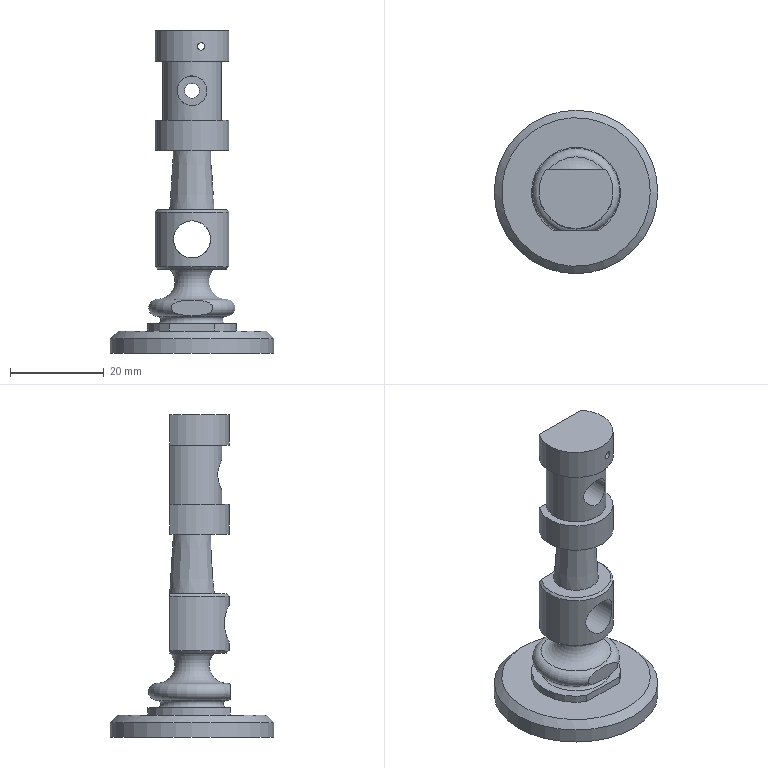Part | NX | features DATUM_CSYS 9, SKETCH 8, EXTRUDE 5, CYLINDER 4, SWP104 3, CHAMFER 2, Intersection Curve 2, CPROJ 1 | 1 solid | 33 faces | box 34.925 x 34.925 x 68.955 mm | volume 12101 mm3 | plane 15 | cylinder 11 | cone 4 | torus 3 | commonest cylinder face diameters 15.875 x3 1.587 x2 3.175 x1 6.35 x1 7.938 x1 12.7 x1
STEP:
#1=CARTESIAN_POINT('',(0.,-7.493,6.35));
#2=VERTEX_POINT('',#1);
#3=CARTESIAN_POINT('',(0.,0.,6.35));
#4=DIRECTION('',(0.,0.,1.));
#5=DIRECTION('',(0.,-1.,0.));
#6=AXIS2_PLACEMENT_3D('',#3,#4,#5);
#7=CIRCLE('',#6,7.493);
#8=EDGE_CURVE('',#2,#2,#7,.T.);
#9=ORIENTED_EDGE('',*,*,#8,.F.);
#10=EDGE_LOOP('',(#9));
#11=FACE_BOUND('',#10,.T.);
#12=CARTESIAN_POINT('',(-4.897,-8.169,6.35));
#13=VERTEX_POINT('',#12);
#14=CARTESIAN_POINT('',(4.897,-8.169,6.35));
#15=VERTEX_POINT('',#14);
#16=CARTESIAN_POINT('',(0.,0.,6.35));
#17=DIRECTION('',(0.,0.,-1.));
#18=DIRECTION('',(1.,0.,0.));
#19=AXIS2_PLACEMENT_3D('',#16,#17,#18);
#20=CIRCLE('',#19,9.525);
#21=EDGE_CURVE('',#13,#15,#20,.T.);
#22=ORIENTED_EDGE('',*,*,#21,.F.);
#23=CARTESIAN_POINT('',(0.,-8.169,6.35));
#24=DIRECTION('',(1.,0.,0.));
#25=VECTOR('',#24,1000.);
#26=LINE('',#23,#25);
#27=EDGE_CURVE('',#13,#15,#26,.T.);
#28=ORIENTED_EDGE('',*,*,#27,.T.);
#29=EDGE_LOOP('',(#22,#28));
#30=FACE_BOUND('',#29,.T.);
#31=CARTESIAN_POINT('',(0.,0.,6.35));
#32=DIRECTION('',(0.,0.,1.));
#33=DIRECTION('',(1.,0.,0.));
#34=AXIS2_PLACEMENT_3D('',#31,#32,#33);
#35=PLANE('',#34);
#36=ADVANCED_FACE('',(#11,#30),#35,.T.);
#37=ORIENTED_EDGE('',*,*,#21,.T.);
#38=CARTESIAN_POINT('',(4.897,-8.169,4.762));
#39=VERTEX_POINT('',#38);
#40=CARTESIAN_POINT('',(4.897,-8.169,4.762));
#41=DIRECTION('',(0.,0.,1.));
#42=VECTOR('',#41,1000.);
#43=LINE('',#40,#42);
#44=EDGE_CURVE('',#15,#39,#43,.F.);
#45=ORIENTED_EDGE('',*,*,#44,.T.);
#46=CARTESIAN_POINT('',(-4.897,-8.169,4.762));
#47=VERTEX_POINT('',#46);
#48=CARTESIAN_POINT('',(0.,0.,4.763));
#49=DIRECTION('',(0.,0.,1.));
#50=DIRECTION('',(1.,0.,0.));
#51=AXIS2_PLACEMENT_3D('',#48,#49,#50);
#52=CIRCLE('',#51,9.525);
#53=EDGE_CURVE('',#39,#47,#52,.T.);
#54=ORIENTED_EDGE('',*,*,#53,.T.);
#55=CARTESIAN_POINT('',(-4.897,-8.169,4.762));
#56=DIRECTION('',(0.,0.,1.));
#57=VECTOR('',#56,1000.);
#58=LINE('',#55,#57);
#59=EDGE_CURVE('',#47,#13,#58,.T.);
#60=ORIENTED_EDGE('',*,*,#59,.T.);
#61=EDGE_LOOP('',(#37,#45,#54,#60));
#62=FACE_BOUND('',#61,.T.);
#63=CARTESIAN_POINT('',(0.,0.,4.763));
#64=DIRECTION('',(0.,0.,1.));
#65=DIRECTION('',(1.,0.,0.));
#66=AXIS2_PLACEMENT_3D('',#63,#64,#65);
#67=CYLINDRICAL_SURFACE('',#66,9.525);
#68=ADVANCED_FACE('',(#62),#67,.T.);
#69=CARTESIAN_POINT('',(0.,-7.493,7.937));
#70=VERTEX_POINT('',#69);
#71=CARTESIAN_POINT('',(0.,0.,7.937));
#72=DIRECTION('',(0.,0.,1.));
#73=DIRECTION('',(0.,-1.,0.));
#74=AXIS2_PLACEMENT_3D('',#71,#72,#73);
#75=CIRCLE('',#74,7.493);
#76=EDGE_CURVE('',#70,#70,#75,.T.);
#77=ORIENTED_EDGE('',*,*,#76,.T.);
#78=EDGE_LOOP('',(#77));
#79=FACE_BOUND('',#78,.T.);
#80=CARTESIAN_POINT('',(0.,7.493,11.537));
#81=VERTEX_POINT('',#80);
#82=CARTESIAN_POINT('',(0.,0.,11.537));
#83=DIRECTION('',(0.,0.,-1.));
#84=DIRECTION('',(0.,1.,0.));
#85=AXIS2_PLACEMENT_3D('',#82,#83,#84);
#86=CIRCLE('',#85,7.493);
#87=EDGE_CURVE('',#81,#81,#86,.T.);
#88=ORIENTED_EDGE('',*,*,#87,.T.);
#89=EDGE_LOOP('',(#88));
#90=FACE_BOUND('',#89,.T.);
#91=CARTESIAN_POINT('',(0.,-8.169,8.069));
#92=VERTEX_POINT('',#91);
#93=CARTESIAN_POINT('',(1.27,-8.169,8.094));
#94=CARTESIAN_POINT('',(0.001629,-8.169,8.057));
#95=CARTESIAN_POINT('',(-1.276,-8.169,8.094));
#96=CARTESIAN_POINT('',(-2.544,-8.169,8.244));
#97=CARTESIAN_POINT('',(-3.572,-8.169,8.567));
#98=CARTESIAN_POINT('',(-4.256,-8.169,9.104));
#99=CARTESIAN_POINT('',(-4.518,-8.169,9.743));
#100=CARTESIAN_POINT('',(-4.25,-8.169,10.378));
#101=CARTESIAN_POINT('',(-3.558,-8.169,10.915));
#102=CARTESIAN_POINT('',(-2.519,-8.169,11.235));
#103=CARTESIAN_POINT('',(-1.257,-8.169,11.382));
#104=CARTESIAN_POINT('',(0.01726,-8.169,11.418));
#105=CARTESIAN_POINT('',(1.296,-8.169,11.38));
#106=CARTESIAN_POINT('',(2.566,-8.169,11.226));
#107=CARTESIAN_POINT('',(3.593,-8.169,10.899));
#108=CARTESIAN_POINT('',(4.27,-8.169,10.352));
#109=CARTESIAN_POINT('',(4.515,-8.169,9.717));
#110=CARTESIAN_POINT('',(4.243,-8.169,9.091));
#111=CARTESIAN_POINT('',(3.558,-8.169,8.562));
#112=CARTESIAN_POINT('',(2.53,-8.169,8.242));
#113=CARTESIAN_POINT('',(1.27,-8.169,8.094));
#114=CARTESIAN_POINT('',(0.001629,-8.169,8.057));
#115=CARTESIAN_POINT('',(-1.276,-8.169,8.094));
#116=B_SPLINE_CURVE_WITH_KNOTS('',3,(#93,#94,#95,#96,#97,#98,#99,#100,#101,#102,#103,#104,#105,#106,#107,#108,#109,#110,#111,#112,#113,#114,#115),.UNSPECIFIED.,.T.,.F.,(1,1,1,1,1,1,1,1,1,1,1,1,1,1,1,1,1,1,1,1,1,1,1,1,1,1,1),(-0.003821,-0.002548,-0.001274,0.,0.001274,0.002548,0.003821,0.004458,0.005095,0.005732,0.006369,0.007643,0.008916,0.01019,0.01146,0.01274,0.01401,0.01465,0.01529,0.01592,0.01656,0.01783,0.01911,0.02038,0.02165,0.02293,0.0242),.UNSPECIFIED.);
#117=EDGE_CURVE('',#92,#92,#116,.T.);
#118=ORIENTED_EDGE('',*,*,#117,.T.);
#119=EDGE_LOOP('',(#118));
#120=FACE_BOUND('',#119,.T.);
#121=CARTESIAN_POINT('',(0.,0.,9.737));
#122=DIRECTION('',(0.,0.,-1.));
#123=DIRECTION('',(0.,1.,0.));
#124=AXIS2_PLACEMENT_3D('',#121,#122,#123);
#125=TOROIDAL_SURFACE('',#124,7.493,1.8);
#126=ADVANCED_FACE('',(#79,#90,#120),#125,.T.);
#127=CARTESIAN_POINT('',(0.,4.763,18.005));
#128=VERTEX_POINT('',#127);
#129=CARTESIAN_POINT('',(5.713,4.763,18.005));
#130=VERTEX_POINT('',#129);
#131=CARTESIAN_POINT('',(0.,4.763,18.005));
#132=DIRECTION('',(1.,0.,0.));
#133=VECTOR('',#132,1000.);
#134=LINE('',#131,#133);
#135=EDGE_CURVE('',#128,#130,#134,.T.);
#136=ORIENTED_EDGE('',*,*,#135,.T.);
#137=CARTESIAN_POINT('',(-5.713,4.763,18.005));
#138=VERTEX_POINT('',#137);
#139=CARTESIAN_POINT('',(0.,0.,18.005));
#140=DIRECTION('',(0.,0.,-1.));
#141=DIRECTION('',(0.,1.,0.));
#142=AXIS2_PLACEMENT_3D('',#139,#140,#141);
#143=CIRCLE('',#142,7.438);
#144=EDGE_CURVE('',#130,#138,#143,.T.);
#145=ORIENTED_EDGE('',*,*,#144,.T.);
#146=CARTESIAN_POINT('',(0.,4.763,18.005));
#147=DIRECTION('',(1.,0.,0.));
#148=VECTOR('',#147,1000.);
#149=LINE('',#146,#148);
#150=EDGE_CURVE('',#138,#128,#149,.T.);
#151=ORIENTED_EDGE('',*,*,#150,.T.);
#152=CARTESIAN_POINT('',(0.,0.,18.005));
#153=DIRECTION('',(0.,0.,1.));
#154=DIRECTION('',(0.,-1.,0.));
#155=AXIS2_PLACEMENT_3D('',#152,#153,#154);
#156=CIRCLE('',#155,4.763);
#157=EDGE_CURVE('',#128,#128,#156,.T.);
#158=ORIENTED_EDGE('',*,*,#157,.T.);
#159=EDGE_LOOP('',(#136,#145,#151,#158));
#160=FACE_BOUND('',#159,.T.);
#161=CARTESIAN_POINT('',(0.,0.,18.005));
#162=DIRECTION('',(0.,0.,-1.));
#163=DIRECTION('',(0.,1.,0.));
#164=AXIS2_PLACEMENT_3D('',#161,#162,#163);
#165=PLANE('',#164);
#166=ADVANCED_FACE('',(#160),#165,.T.);
#167=CARTESIAN_POINT('',(0.,-7.938,28.323));
#168=VERTEX_POINT('',#167);
#169=CARTESIAN_POINT('',(3.118,-7.441,27.461));
#170=CARTESIAN_POINT('',(-0.001391,-8.185,28.755));
#171=CARTESIAN_POINT('',(-3.112,-7.443,27.458));
#172=CARTESIAN_POINT('',(-4.396,-6.59,24.369));
#173=CARTESIAN_POINT('',(-3.115,-7.44,21.25));
#174=CARTESIAN_POINT('',(-0.01564,-8.185,19.955));
#175=CARTESIAN_POINT('',(3.112,-7.445,21.246));
#176=CARTESIAN_POINT('',(4.396,-6.59,24.34));
#177=CARTESIAN_POINT('',(3.118,-7.441,27.461));
#178=CARTESIAN_POINT('',(-0.001391,-8.185,28.755));
#179=CARTESIAN_POINT('',(-3.112,-7.443,27.458));
#180=B_SPLINE_CURVE_WITH_KNOTS('',3,(#169,#170,#171,#172,#173,#174,#175,#176,#177,#178,#179),.UNSPECIFIED.,.T.,.F.,(1,1,1,1,1,1,1,1,1,1,1,1,1,1,1),(-0.00946,-0.006307,-0.003153,0.,0.003153,0.006307,0.00946,0.01261,0.01577,0.01892,0.02207,0.02523,0.02838,0.03153,0.03469),.UNSPECIFIED.);
#181=EDGE_CURVE('',#168,#168,#180,.T.);
#182=ORIENTED_EDGE('',*,*,#181,.F.);
#183=EDGE_LOOP('',(#182));
#184=FACE_BOUND('',#183,.T.);
#185=CARTESIAN_POINT('',(-6.35,4.763,30.205));
#186=VERTEX_POINT('',#185);
#187=CARTESIAN_POINT('',(-6.35,4.762,18.505));
#188=VERTEX_POINT('',#187);
#189=CARTESIAN_POINT('',(-6.35,4.763,43.405));
#190=DIRECTION('',(0.,0.,-1.));
#191=VECTOR('',#190,1000.);
#192=LINE('',#189,#191);
#193=EDGE_CURVE('',#186,#188,#192,.T.);
#194=ORIENTED_EDGE('',*,*,#193,.T.);
#195=CARTESIAN_POINT('',(6.35,4.762,18.505));
#196=VERTEX_POINT('',#195);
#197=CARTESIAN_POINT('',(0.,0.,18.505));
#198=DIRECTION('',(0.,0.,-1.));
#199=DIRECTION('',(0.,1.,0.));
#200=AXIS2_PLACEMENT_3D('',#197,#198,#199);
#201=CIRCLE('',#200,7.938);
#202=EDGE_CURVE('',#188,#196,#201,.F.);
#203=ORIENTED_EDGE('',*,*,#202,.T.);
#204=CARTESIAN_POINT('',(6.35,4.763,30.205));
#205=VERTEX_POINT('',#204);
#206=CARTESIAN_POINT('',(6.35,4.763,43.405));
#207=DIRECTION('',(0.,0.,-1.));
#208=VECTOR('',#207,1000.);
#209=LINE('',#206,#208);
#210=EDGE_CURVE('',#196,#205,#209,.F.);
#211=ORIENTED_EDGE('',*,*,#210,.T.);
#212=CARTESIAN_POINT('',(0.,0.,30.205));
#213=DIRECTION('',(0.,0.,1.));
#214=DIRECTION('',(0.,-1.,0.));
#215=AXIS2_PLACEMENT_3D('',#212,#213,#214);
#216=CIRCLE('',#215,7.938);
#217=EDGE_CURVE('',#205,#186,#216,.F.);
#218=ORIENTED_EDGE('',*,*,#217,.T.);
#219=EDGE_LOOP('',(#194,#203,#211,#218));
#220=FACE_BOUND('',#219,.T.);
#221=CARTESIAN_POINT('',(0.,0.,43.405));
#222=DIRECTION('',(0.,0.,-1.));
#223=DIRECTION('',(0.,1.,0.));
#224=AXIS2_PLACEMENT_3D('',#221,#222,#223);
#225=CYLINDRICAL_SURFACE('',#224,7.938);
#226=ADVANCED_FACE('',(#184,#220),#225,.T.);
#227=CARTESIAN_POINT('',(0.,4.763,30.705));
#228=VERTEX_POINT('',#227);
#229=CARTESIAN_POINT('',(-5.713,4.763,30.705));
#230=VERTEX_POINT('',#229);
#231=CARTESIAN_POINT('',(0.,4.763,30.705));
#232=DIRECTION('',(-1.,0.,0.));
#233=VECTOR('',#232,1000.);
#234=LINE('',#231,#233);
#235=EDGE_CURVE('',#228,#230,#234,.T.);
#236=ORIENTED_EDGE('',*,*,#235,.T.);
#237=CARTESIAN_POINT('',(5.713,4.763,30.705));
#238=VERTEX_POINT('',#237);
#239=CARTESIAN_POINT('',(0.,0.,30.705));
#240=DIRECTION('',(0.,0.,1.));
#241=DIRECTION('',(0.,-1.,0.));
#242=AXIS2_PLACEMENT_3D('',#239,#240,#241);
#243=CIRCLE('',#242,7.438);
#244=EDGE_CURVE('',#230,#238,#243,.T.);
#245=ORIENTED_EDGE('',*,*,#244,.T.);
#246=CARTESIAN_POINT('',(0.,4.763,30.705));
#247=DIRECTION('',(-1.,0.,0.));
#248=VECTOR('',#247,1000.);
#249=LINE('',#246,#248);
#250=EDGE_CURVE('',#238,#228,#249,.T.);
#251=ORIENTED_EDGE('',*,*,#250,.T.);
#252=CARTESIAN_POINT('',(0.,0.,30.705));
#253=DIRECTION('',(0.,0.,-1.));
#254=DIRECTION('',(0.,1.,0.));
#255=AXIS2_PLACEMENT_3D('',#252,#253,#254);
#256=CIRCLE('',#255,4.763);
#257=EDGE_CURVE('',#228,#228,#256,.T.);
#258=ORIENTED_EDGE('',*,*,#257,.T.);
#259=EDGE_LOOP('',(#236,#245,#251,#258));
#260=FACE_BOUND('',#259,.T.);
#261=CARTESIAN_POINT('',(0.,7.938,30.705));
#262=DIRECTION('',(0.,0.,1.));
#263=DIRECTION('',(0.,-1.,0.));
#264=AXIS2_PLACEMENT_3D('',#261,#262,#263);
#265=PLANE('',#264);
#266=ADVANCED_FACE('',(#260),#265,.T.);
#267=CARTESIAN_POINT('',(0.,3.969,43.405));
#268=VERTEX_POINT('',#267);
#269=CARTESIAN_POINT('',(0.,0.,43.405));
#270=DIRECTION('',(0.,0.,-1.));
#271=DIRECTION('',(0.,1.,0.));
#272=AXIS2_PLACEMENT_3D('',#269,#270,#271);
#273=CIRCLE('',#272,3.969);
#274=EDGE_CURVE('',#268,#268,#273,.T.);
#275=ORIENTED_EDGE('',*,*,#274,.F.);
#276=EDGE_LOOP('',(#275));
#277=FACE_BOUND('',#276,.T.);
#278=CARTESIAN_POINT('',(6.35,4.763,43.405));
#279=VERTEX_POINT('',#278);
#280=CARTESIAN_POINT('',(-6.35,4.763,43.405));
#281=VERTEX_POINT('',#280);
#282=CARTESIAN_POINT('',(0.,0.,43.405));
#283=DIRECTION('',(0.,0.,-1.));
#284=DIRECTION('',(0.,1.,0.));
#285=AXIS2_PLACEMENT_3D('',#282,#283,#284);
#286=CIRCLE('',#285,7.938);
#287=EDGE_CURVE('',#279,#281,#286,.T.);
#288=ORIENTED_EDGE('',*,*,#287,.T.);
#289=CARTESIAN_POINT('',(0.,4.763,43.405));
#290=DIRECTION('',(1.,0.,0.));
#291=VECTOR('',#290,1000.);
#292=LINE('',#289,#291);
#293=EDGE_CURVE('',#281,#279,#292,.T.);
#294=ORIENTED_EDGE('',*,*,#293,.T.);
#295=EDGE_LOOP('',(#288,#294));
#296=FACE_BOUND('',#295,.T.);
#297=CARTESIAN_POINT('',(0.,3.969,43.405));
#298=DIRECTION('',(0.,0.,-1.));
#299=DIRECTION('',(0.,1.,0.));
#300=AXIS2_PLACEMENT_3D('',#297,#298,#299);
#301=PLANE('',#300);
#302=ADVANCED_FACE('',(#277,#296),#301,.T.);
#303=ORIENTED_EDGE('',*,*,#287,.F.);
#304=CARTESIAN_POINT('',(6.35,4.762,49.755));
#305=VERTEX_POINT('',#304);
#306=CARTESIAN_POINT('',(6.35,4.763,43.405));
#307=DIRECTION('',(0.,0.,-1.));
#308=VECTOR('',#307,1000.);
#309=LINE('',#306,#308);
#310=EDGE_CURVE('',#279,#305,#309,.F.);
#311=ORIENTED_EDGE('',*,*,#310,.T.);
#312=CARTESIAN_POINT('',(-6.35,4.762,49.755));
#313=VERTEX_POINT('',#312);
#314=CARTESIAN_POINT('',(0.,0.,49.755));
#315=DIRECTION('',(0.,0.,-1.));
#316=DIRECTION('',(0.,1.,0.));
#317=AXIS2_PLACEMENT_3D('',#314,#315,#316);
#318=CIRCLE('',#317,7.938);
#319=EDGE_CURVE('',#305,#313,#318,.T.);
#320=ORIENTED_EDGE('',*,*,#319,.T.);
#321=CARTESIAN_POINT('',(-6.35,4.763,43.405));
#322=DIRECTION('',(0.,0.,-1.));
#323=VECTOR('',#322,1000.);
#324=LINE('',#321,#323);
#325=EDGE_CURVE('',#313,#281,#324,.T.);
#326=ORIENTED_EDGE('',*,*,#325,.T.);
#327=EDGE_LOOP('',(#303,#311,#320,#326));
#328=FACE_BOUND('',#327,.T.);
#329=CARTESIAN_POINT('',(0.,0.,43.405));
#330=DIRECTION('',(0.,0.,-1.));
#331=DIRECTION('',(0.,1.,0.));
#332=AXIS2_PLACEMENT_3D('',#329,#330,#331);
#333=CYLINDRICAL_SURFACE('',#332,7.938);
#334=ADVANCED_FACE('',(#328),#333,.T.);
#335=ORIENTED_EDGE('',*,*,#319,.F.);
#336=CARTESIAN_POINT('',(4.2,4.763,49.755));
#337=VERTEX_POINT('',#336);
#338=CARTESIAN_POINT('',(0.,4.762,49.755));
#339=DIRECTION('',(-1.,0.,0.));
#340=VECTOR('',#339,1000.);
#341=LINE('',#338,#340);
#342=EDGE_CURVE('',#305,#337,#341,.T.);
#343=ORIENTED_EDGE('',*,*,#342,.T.);
#344=CARTESIAN_POINT('',(-4.2,4.763,49.755));
#345=VERTEX_POINT('',#344);
#346=CARTESIAN_POINT('',(0.,0.,49.755));
#347=DIRECTION('',(0.,0.,-1.));
#348=DIRECTION('',(0.,1.,0.));
#349=AXIS2_PLACEMENT_3D('',#346,#347,#348);
#350=CIRCLE('',#349,6.35);
#351=EDGE_CURVE('',#337,#345,#350,.T.);
#352=ORIENTED_EDGE('',*,*,#351,.T.);
#353=CARTESIAN_POINT('',(0.,4.762,49.755));
#354=DIRECTION('',(-1.,0.,0.));
#355=VECTOR('',#354,1000.);
#356=LINE('',#353,#355);
#357=EDGE_CURVE('',#345,#313,#356,.T.);
#358=ORIENTED_EDGE('',*,*,#357,.T.);
#359=EDGE_LOOP('',(#335,#343,#352,#358));
#360=FACE_BOUND('',#359,.T.);
#361=CARTESIAN_POINT('',(0.,7.938,49.755));
#362=DIRECTION('',(0.,0.,1.));
#363=DIRECTION('',(0.,-1.,0.));
#364=AXIS2_PLACEMENT_3D('',#361,#362,#363);
#365=PLANE('',#364);
#366=ADVANCED_FACE('',(#360),#365,.T.);
#367=CARTESIAN_POINT('',(3.175,-5.499,56.105));
#368=VERTEX_POINT('',#367);
#369=CARTESIAN_POINT('',(2.491,-5.955,53.617));
#370=CARTESIAN_POINT('',(3.517,-5.272,56.106));
#371=CARTESIAN_POINT('',(2.489,-5.954,58.588));
#372=CARTESIAN_POINT('',(0.009887,-6.548,59.625));
#373=CARTESIAN_POINT('',(-2.49,-5.955,58.59));
#374=CARTESIAN_POINT('',(-3.517,-5.272,56.117));
#375=CARTESIAN_POINT('',(-2.493,-5.952,53.621));
#376=CARTESIAN_POINT('',(-0.01032,-6.548,52.585));
#377=CARTESIAN_POINT('',(2.491,-5.955,53.617));
#378=CARTESIAN_POINT('',(3.517,-5.272,56.106));
#379=CARTESIAN_POINT('',(2.489,-5.954,58.588));
#380=B_SPLINE_CURVE_WITH_KNOTS('',3,(#369,#370,#371,#372,#373,#374,#375,#376,#377,#378,#379),.UNSPECIFIED.,.T.,.F.,(1,1,1,1,1,1,1,1,1,1,1,1,1,1,1),(-0.007567,-0.005045,-0.002522,0.,0.002522,0.005045,0.007567,0.01009,0.01261,0.01513,0.01766,0.02018,0.0227,0.02522,0.02775),.UNSPECIFIED.);
#381=EDGE_CURVE('',#368,#368,#380,.T.);
#382=ORIENTED_EDGE('',*,*,#381,.F.);
#383=EDGE_LOOP('',(#382));
#384=FACE_BOUND('',#383,.T.);
#385=ORIENTED_EDGE('',*,*,#351,.F.);
#386=CARTESIAN_POINT('',(4.2,4.762,62.455));
#387=VERTEX_POINT('',#386);
#388=CARTESIAN_POINT('',(4.2,4.763,43.405));
#389=DIRECTION('',(0.,0.,-1.));
#390=VECTOR('',#389,1000.);
#391=LINE('',#388,#390);
#392=EDGE_CURVE('',#337,#387,#391,.F.);
#393=ORIENTED_EDGE('',*,*,#392,.T.);
#394=CARTESIAN_POINT('',(-4.2,4.762,62.455));
#395=VERTEX_POINT('',#394);
#396=CARTESIAN_POINT('',(0.,0.,62.455));
#397=DIRECTION('',(0.,0.,-1.));
#398=DIRECTION('',(0.,1.,0.));
#399=AXIS2_PLACEMENT_3D('',#396,#397,#398);
#400=CIRCLE('',#399,6.35);
#401=EDGE_CURVE('',#387,#395,#400,.T.);
#402=ORIENTED_EDGE('',*,*,#401,.T.);
#403=CARTESIAN_POINT('',(-4.2,4.763,43.405));
#404=DIRECTION('',(0.,0.,-1.));
#405=VECTOR('',#404,1000.);
#406=LINE('',#403,#405);
#407=EDGE_CURVE('',#395,#345,#406,.T.);
#408=ORIENTED_EDGE('',*,*,#407,.T.);
#409=EDGE_LOOP('',(#385,#393,#402,#408));
#410=FACE_BOUND('',#409,.T.);
#411=CARTESIAN_POINT('',(0.,0.,43.405));
#412=DIRECTION('',(0.,0.,-1.));
#413=DIRECTION('',(0.,1.,0.));
#414=AXIS2_PLACEMENT_3D('',#411,#412,#413);
#415=CYLINDRICAL_SURFACE('',#414,6.35);
#416=ADVANCED_FACE('',(#384,#410),#415,.T.);
#417=CARTESIAN_POINT('',(6.35,4.763,62.455));
#418=VERTEX_POINT('',#417);
#419=CARTESIAN_POINT('',(-6.35,4.763,62.455));
#420=VERTEX_POINT('',#419);
#421=CARTESIAN_POINT('',(0.,0.,62.455));
#422=DIRECTION('',(0.,0.,-1.));
#423=DIRECTION('',(0.,1.,0.));
#424=AXIS2_PLACEMENT_3D('',#421,#422,#423);
#425=CIRCLE('',#424,7.938);
#426=EDGE_CURVE('',#418,#420,#425,.T.);
#427=ORIENTED_EDGE('',*,*,#426,.T.);
#428=CARTESIAN_POINT('',(0.,4.762,62.455));
#429=DIRECTION('',(1.,0.,0.));
#430=VECTOR('',#429,1000.);
#431=LINE('',#428,#430);
#432=EDGE_CURVE('',#420,#395,#431,.T.);
#433=ORIENTED_EDGE('',*,*,#432,.T.);
#434=ORIENTED_EDGE('',*,*,#401,.F.);
#435=CARTESIAN_POINT('',(0.,4.762,62.455));
#436=DIRECTION('',(1.,0.,0.));
#437=VECTOR('',#436,1000.);
#438=LINE('',#435,#437);
#439=EDGE_CURVE('',#387,#418,#438,.T.);
#440=ORIENTED_EDGE('',*,*,#439,.T.);
#441=EDGE_LOOP('',(#427,#433,#434,#440));
#442=FACE_BOUND('',#441,.T.);
#443=CARTESIAN_POINT('',(0.,6.35,62.455));
#444=DIRECTION('',(0.,0.,-1.));
#445=DIRECTION('',(0.,1.,0.));
#446=AXIS2_PLACEMENT_3D('',#443,#444,#445);
#447=PLANE('',#446);
#448=ADVANCED_FACE('',(#442),#447,.T.);
#449=CARTESIAN_POINT('',(1.903,-7.706,66.381));
#450=VERTEX_POINT('',#449);
#451=CARTESIAN_POINT('',(2.515,-7.534,66.216));
#452=CARTESIAN_POINT('',(1.694,-7.779,66.558));
#453=CARTESIAN_POINT('',(0.9196,-7.885,65.803));
#454=CARTESIAN_POINT('',(1.295,-7.836,64.948));
#455=CARTESIAN_POINT('',(1.92,-7.712,64.712));
#456=CARTESIAN_POINT('',(2.523,-7.531,64.965));
#457=CARTESIAN_POINT('',(2.786,-7.432,65.594));
#458=CARTESIAN_POINT('',(2.515,-7.534,66.216));
#459=CARTESIAN_POINT('',(1.694,-7.779,66.558));
#460=CARTESIAN_POINT('',(0.9196,-7.885,65.803));
#461=B_SPLINE_CURVE_WITH_KNOTS('',3,(#451,#452,#453,#454,#455,#456,#457,#458,#459,#460),.UNSPECIFIED.,.T.,.F.,(1,1,1,1,1,1,1,1,1,1,1,1,1,1),(-0.00189,-0.00126,-0.0006301,0.,0.00126,0.00189,0.00252,0.003151,0.003781,0.004411,0.005041,0.006301,0.006931,0.007561),.UNSPECIFIED.);
#462=EDGE_CURVE('',#450,#450,#461,.T.);
#463=ORIENTED_EDGE('',*,*,#462,.F.);
#464=EDGE_LOOP('',(#463));
#465=FACE_BOUND('',#464,.T.);
#466=ORIENTED_EDGE('',*,*,#426,.F.);
#467=CARTESIAN_POINT('',(6.35,4.762,68.955));
#468=VERTEX_POINT('',#467);
#469=CARTESIAN_POINT('',(6.35,4.763,43.405));
#470=DIRECTION('',(0.,0.,-1.));
#471=VECTOR('',#470,1000.);
#472=LINE('',#469,#471);
#473=EDGE_CURVE('',#418,#468,#472,.F.);
#474=ORIENTED_EDGE('',*,*,#473,.T.);
#475=CARTESIAN_POINT('',(-6.35,4.762,68.955));
#476=VERTEX_POINT('',#475);
#477=CARTESIAN_POINT('',(0.,0.,68.955));
#478=DIRECTION('',(0.,0.,-1.));
#479=DIRECTION('',(0.,1.,0.));
#480=AXIS2_PLACEMENT_3D('',#477,#478,#479);
#481=CIRCLE('',#480,7.938);
#482=EDGE_CURVE('',#468,#476,#481,.T.);
#483=ORIENTED_EDGE('',*,*,#482,.T.);
#484=CARTESIAN_POINT('',(-6.35,4.763,43.405));
#485=DIRECTION('',(0.,0.,-1.));
#486=VECTOR('',#485,1000.);
#487=LINE('',#484,#486);
#488=EDGE_CURVE('',#476,#420,#487,.T.);
#489=ORIENTED_EDGE('',*,*,#488,.T.);
#490=EDGE_LOOP('',(#466,#474,#483,#489));
#491=FACE_BOUND('',#490,.T.);
#492=CARTESIAN_POINT('',(0.,0.,43.405));
#493=DIRECTION('',(0.,0.,-1.));
#494=DIRECTION('',(0.,1.,0.));
#495=AXIS2_PLACEMENT_3D('',#492,#493,#494);
#496=CYLINDRICAL_SURFACE('',#495,7.938);
#497=ADVANCED_FACE('',(#465,#491),#496,.T.);
#498=ORIENTED_EDGE('',*,*,#482,.F.);
#499=CARTESIAN_POINT('',(0.,4.762,68.955));
#500=DIRECTION('',(-1.,0.,0.));
#501=VECTOR('',#500,1000.);
#502=LINE('',#499,#501);
#503=EDGE_CURVE('',#468,#476,#502,.T.);
#504=ORIENTED_EDGE('',*,*,#503,.T.);
#505=EDGE_LOOP('',(#498,#504));
#506=FACE_BOUND('',#505,.T.);
#507=CARTESIAN_POINT('',(0.,7.938,68.955));
#508=DIRECTION('',(0.,0.,1.));
#509=DIRECTION('',(0.,-1.,0.));
#510=AXIS2_PLACEMENT_3D('',#507,#508,#509);
#511=PLANE('',#510);
#512=ADVANCED_FACE('',(#506),#511,.T.);
#513=ORIENTED_EDGE('',*,*,#53,.F.);
#514=CARTESIAN_POINT('',(22.,-8.169,4.762));
#515=DIRECTION('',(-1.,0.,0.));
#516=VECTOR('',#515,1000.);
#517=LINE('',#514,#516);
#518=EDGE_CURVE('',#39,#47,#517,.T.);
#519=ORIENTED_EDGE('',*,*,#518,.T.);
#520=EDGE_LOOP('',(#513,#519));
#521=FACE_BOUND('',#520,.T.);
#522=CARTESIAN_POINT('',(15.875,0.,4.763));
#523=VERTEX_POINT('',#522);
#524=CARTESIAN_POINT('',(0.,0.,4.763));
#525=DIRECTION('',(0.,0.,1.));
#526=DIRECTION('',(1.,0.,0.));
#527=AXIS2_PLACEMENT_3D('',#524,#525,#526);
#528=CIRCLE('',#527,15.875);
#529=EDGE_CURVE('',#523,#523,#528,.T.);
#530=ORIENTED_EDGE('',*,*,#529,.T.);
#531=EDGE_LOOP('',(#530));
#532=FACE_BOUND('',#531,.T.);
#533=CARTESIAN_POINT('',(0.,0.,4.763));
#534=DIRECTION('',(0.,0.,1.));
#535=DIRECTION('',(1.,0.,0.));
#536=AXIS2_PLACEMENT_3D('',#533,#534,#535);
#537=PLANE('',#536);
#538=ADVANCED_FACE('',(#521,#532),#537,.T.);
#539=CARTESIAN_POINT('',(17.462,0.,0.));
#540=VERTEX_POINT('',#539);
#541=CARTESIAN_POINT('',(0.,0.,0.));
#542=DIRECTION('',(0.,0.,1.));
#543=DIRECTION('',(1.,0.,0.));
#544=AXIS2_PLACEMENT_3D('',#541,#542,#543);
#545=CIRCLE('',#544,17.462);
#546=EDGE_CURVE('',#540,#540,#545,.T.);
#547=ORIENTED_EDGE('',*,*,#546,.F.);
#548=EDGE_LOOP('',(#547));
#549=FACE_BOUND('',#548,.T.);
#550=CARTESIAN_POINT('',(0.,0.,0.));
#551=DIRECTION('',(0.,0.,-1.));
#552=DIRECTION('',(-1.,0.,0.));
#553=AXIS2_PLACEMENT_3D('',#550,#551,#552);
#554=PLANE('',#553);
#555=ADVANCED_FACE('',(#549),#554,.T.);
#556=CARTESIAN_POINT('',(17.462,0.,3.175));
#557=VERTEX_POINT('',#556);
#558=CARTESIAN_POINT('',(0.,0.,3.175));
#559=DIRECTION('',(0.,0.,1.));
#560=DIRECTION('',(1.,0.,0.));
#561=AXIS2_PLACEMENT_3D('',#558,#559,#560);
#562=CIRCLE('',#561,17.462);
#563=EDGE_CURVE('',#557,#557,#562,.F.);
#564=ORIENTED_EDGE('',*,*,#563,.T.);
#565=EDGE_LOOP('',(#564));
#566=FACE_BOUND('',#565,.T.);
#567=ORIENTED_EDGE('',*,*,#546,.T.);
#568=EDGE_LOOP('',(#567));
#569=FACE_BOUND('',#568,.T.);
#570=CARTESIAN_POINT('',(0.,0.,0.));
#571=DIRECTION('',(0.,0.,1.));
#572=DIRECTION('',(1.,0.,0.));
#573=AXIS2_PLACEMENT_3D('',#570,#571,#572);
#574=CYLINDRICAL_SURFACE('',#573,17.462);
#575=ADVANCED_FACE('',(#566,#569),#574,.T.);
#576=ORIENTED_EDGE('',*,*,#529,.F.);
#577=EDGE_LOOP('',(#576));
#578=FACE_BOUND('',#577,.T.);
#579=ORIENTED_EDGE('',*,*,#563,.F.);
#580=EDGE_LOOP('',(#579));
#581=FACE_BOUND('',#580,.T.);
#582=CARTESIAN_POINT('',(0.,0.,3.175));
#583=DIRECTION('',(0.,0.,-1.));
#584=DIRECTION('',(-1.,0.,0.));
#585=AXIS2_PLACEMENT_3D('',#582,#583,#584);
#586=CONICAL_SURFACE('',#585,17.462,0.7854);
#587=ADVANCED_FACE('',(#578,#581),#586,.T.);
#588=ORIENTED_EDGE('',*,*,#76,.F.);
#589=EDGE_LOOP('',(#588));
#590=FACE_BOUND('',#589,.T.);
#591=ORIENTED_EDGE('',*,*,#8,.T.);
#592=EDGE_LOOP('',(#591));
#593=FACE_BOUND('',#592,.T.);
#594=CARTESIAN_POINT('',(0.,0.,7.144));
#595=DIRECTION('',(0.,0.,1.));
#596=DIRECTION('',(0.,-1.,0.));
#597=AXIS2_PLACEMENT_3D('',#594,#595,#596);
#598=TOROIDAL_SURFACE('',#597,7.493,0.7937);
#599=ADVANCED_FACE('',(#590,#593),#598,.F.);
#600=ORIENTED_EDGE('',*,*,#157,.F.);
#601=EDGE_LOOP('',(#600));
#602=FACE_BOUND('',#601,.T.);
#603=ORIENTED_EDGE('',*,*,#87,.F.);
#604=EDGE_LOOP('',(#603));
#605=FACE_BOUND('',#604,.T.);
#606=CARTESIAN_POINT('',(0.,0.,15.347));
#607=DIRECTION('',(0.,0.,-1.));
#608=DIRECTION('',(0.,1.,0.));
#609=AXIS2_PLACEMENT_3D('',#606,#607,#608);
#610=TOROIDAL_SURFACE('',#609,7.493,3.81);
#611=ADVANCED_FACE('',(#602,#605),#610,.F.);
#612=ORIENTED_EDGE('',*,*,#274,.T.);
#613=EDGE_LOOP('',(#612));
#614=FACE_BOUND('',#613,.T.);
#615=ORIENTED_EDGE('',*,*,#257,.F.);
#616=EDGE_LOOP('',(#615));
#617=FACE_BOUND('',#616,.T.);
#618=CARTESIAN_POINT('',(0.,0.,30.705));
#619=DIRECTION('',(0.,0.,-1.));
#620=DIRECTION('',(0.,1.,0.));
#621=AXIS2_PLACEMENT_3D('',#618,#619,#620);
#622=CONICAL_SURFACE('',#621,4.763,0.06242);
#623=ADVANCED_FACE('',(#614,#617),#622,.T.);
#624=CARTESIAN_POINT('',(-2.697,4.762,65.587));
#625=VERTEX_POINT('',#624);
#626=CARTESIAN_POINT('',(-1.903,4.762,65.587));
#627=DIRECTION('',(0.,1.,0.));
#628=DIRECTION('',(-1.,0.,0.));
#629=AXIS2_PLACEMENT_3D('',#626,#627,#628);
#630=CIRCLE('',#629,0.7937);
#631=EDGE_CURVE('',#625,#625,#630,.T.);
#632=ORIENTED_EDGE('',*,*,#631,.F.);
#633=EDGE_LOOP('',(#632));
#634=FACE_BOUND('',#633,.T.);
#635=CARTESIAN_POINT('',(1.109,4.762,65.587));
#636=VERTEX_POINT('',#635);
#637=CARTESIAN_POINT('',(1.903,4.762,65.587));
#638=DIRECTION('',(0.,1.,0.));
#639=DIRECTION('',(-1.,0.,0.));
#640=AXIS2_PLACEMENT_3D('',#637,#638,#639);
#641=CIRCLE('',#640,0.7937);
#642=EDGE_CURVE('',#636,#636,#641,.T.);
#643=ORIENTED_EDGE('',*,*,#642,.F.);
#644=EDGE_LOOP('',(#643));
#645=FACE_BOUND('',#644,.T.);
#646=CARTESIAN_POINT('',(1.587,4.762,56.105));
#647=VERTEX_POINT('',#646);
#648=CARTESIAN_POINT('',(0.,4.762,56.105));
#649=DIRECTION('',(0.,-1.,0.));
#650=DIRECTION('',(1.,0.,0.));
#651=AXIS2_PLACEMENT_3D('',#648,#649,#650);
#652=CIRCLE('',#651,1.587);
#653=EDGE_CURVE('',#647,#647,#652,.T.);
#654=ORIENTED_EDGE('',*,*,#653,.T.);
#655=EDGE_LOOP('',(#654));
#656=FACE_BOUND('',#655,.T.);
#657=ORIENTED_EDGE('',*,*,#325,.F.);
#658=ORIENTED_EDGE('',*,*,#357,.F.);
#659=ORIENTED_EDGE('',*,*,#407,.F.);
#660=ORIENTED_EDGE('',*,*,#432,.F.);
#661=ORIENTED_EDGE('',*,*,#488,.F.);
#662=ORIENTED_EDGE('',*,*,#503,.F.);
#663=ORIENTED_EDGE('',*,*,#473,.F.);
#664=ORIENTED_EDGE('',*,*,#439,.F.);
#665=ORIENTED_EDGE('',*,*,#392,.F.);
#666=ORIENTED_EDGE('',*,*,#342,.F.);
#667=ORIENTED_EDGE('',*,*,#310,.F.);
#668=ORIENTED_EDGE('',*,*,#293,.F.);
#669=EDGE_LOOP('',(#657,#658,#659,#660,#661,#662,#663,#664,#665,#666,#667,#668));
#670=FACE_BOUND('',#669,.T.);
#671=CARTESIAN_POINT('',(22.,4.762,73.386));
#672=DIRECTION('',(0.,1.,0.));
#673=DIRECTION('',(0.,0.,1.));
#674=AXIS2_PLACEMENT_3D('',#671,#672,#673);
#675=PLANE('',#674);
#676=ADVANCED_FACE('',(#634,#645,#656,#670),#675,.T.);
#677=CARTESIAN_POINT('',(-3.969,4.763,24.355));
#678=VERTEX_POINT('',#677);
#679=CARTESIAN_POINT('',(0.,4.763,24.355));
#680=DIRECTION('',(0.,1.,0.));
#681=DIRECTION('',(-1.,0.,0.));
#682=AXIS2_PLACEMENT_3D('',#679,#680,#681);
#683=CIRCLE('',#682,3.969);
#684=EDGE_CURVE('',#678,#678,#683,.T.);
#685=ORIENTED_EDGE('',*,*,#684,.F.);
#686=EDGE_LOOP('',(#685));
#687=FACE_BOUND('',#686,.T.);
#688=ORIENTED_EDGE('',*,*,#150,.F.);
#689=CARTESIAN_POINT('',(-5.713,4.763,18.005));
#690=CARTESIAN_POINT('',(-5.927,4.763,18.169));
#691=CARTESIAN_POINT('',(-6.139,4.763,18.336));
#692=CARTESIAN_POINT('',(-6.35,4.763,18.505));
#693=B_SPLINE_CURVE_WITH_KNOTS('',3,(#689,#690,#691,#692),.UNSPECIFIED.,.F.,.F.,(4,4),(0.,0.00081),.UNSPECIFIED.);
#694=EDGE_CURVE('',#138,#188,#693,.T.);
#695=ORIENTED_EDGE('',*,*,#694,.T.);
#696=ORIENTED_EDGE('',*,*,#193,.F.);
#697=CARTESIAN_POINT('',(-6.35,4.762,30.205));
#698=CARTESIAN_POINT('',(-6.139,4.762,30.373));
#699=CARTESIAN_POINT('',(-5.927,4.763,30.54));
#700=CARTESIAN_POINT('',(-5.713,4.763,30.705));
#701=B_SPLINE_CURVE_WITH_KNOTS('',3,(#697,#698,#699,#700),.UNSPECIFIED.,.F.,.F.,(4,4),(0.,0.00081),.UNSPECIFIED.);
#702=EDGE_CURVE('',#186,#230,#701,.T.);
#703=ORIENTED_EDGE('',*,*,#702,.T.);
#704=ORIENTED_EDGE('',*,*,#235,.F.);
#705=ORIENTED_EDGE('',*,*,#250,.F.);
#706=CARTESIAN_POINT('',(5.713,4.763,30.705));
#707=CARTESIAN_POINT('',(5.927,4.763,30.54));
#708=CARTESIAN_POINT('',(6.139,4.763,30.373));
#709=CARTESIAN_POINT('',(6.35,4.763,30.205));
#710=B_SPLINE_CURVE_WITH_KNOTS('',3,(#706,#707,#708,#709),.UNSPECIFIED.,.F.,.F.,(4,4),(0.,0.00081),.UNSPECIFIED.);
#711=EDGE_CURVE('',#238,#205,#710,.T.);
#712=ORIENTED_EDGE('',*,*,#711,.T.);
#713=ORIENTED_EDGE('',*,*,#210,.F.);
#714=CARTESIAN_POINT('',(6.35,4.762,18.505));
#715=CARTESIAN_POINT('',(6.139,4.762,18.336));
#716=CARTESIAN_POINT('',(5.927,4.763,18.169));
#717=CARTESIAN_POINT('',(5.713,4.763,18.005));
#718=B_SPLINE_CURVE_WITH_KNOTS('',3,(#714,#715,#716,#717),.UNSPECIFIED.,.F.,.F.,(4,4),(0.,0.00081),.UNSPECIFIED.);
#719=EDGE_CURVE('',#196,#130,#718,.T.);
#720=ORIENTED_EDGE('',*,*,#719,.T.);
#721=ORIENTED_EDGE('',*,*,#135,.F.);
#722=EDGE_LOOP('',(#688,#695,#696,#703,#704,#705,#712,#713,#720,#721));
#723=FACE_BOUND('',#722,.T.);
#724=CARTESIAN_POINT('',(22.,4.762,73.386));
#725=DIRECTION('',(0.,1.,0.));
#726=DIRECTION('',(0.,0.,1.));
#727=AXIS2_PLACEMENT_3D('',#724,#725,#726);
#728=PLANE('',#727);
#729=ADVANCED_FACE('',(#687,#723),#728,.T.);
#730=ORIENTED_EDGE('',*,*,#117,.F.);
#731=EDGE_LOOP('',(#730));
#732=FACE_BOUND('',#731,.T.);
#733=CARTESIAN_POINT('',(22.,-8.169,4.762));
#734=DIRECTION('',(0.,-1.,0.));
#735=DIRECTION('',(0.,0.,-1.));
#736=AXIS2_PLACEMENT_3D('',#733,#734,#735);
#737=PLANE('',#736);
#738=ADVANCED_FACE('',(#732),#737,.T.);
#739=ORIENTED_EDGE('',*,*,#27,.F.);
#740=ORIENTED_EDGE('',*,*,#59,.F.);
#741=ORIENTED_EDGE('',*,*,#518,.F.);
#742=ORIENTED_EDGE('',*,*,#44,.F.);
#743=EDGE_LOOP('',(#739,#740,#741,#742));
#744=FACE_BOUND('',#743,.T.);
#745=CARTESIAN_POINT('',(22.,-8.169,4.762));
#746=DIRECTION('',(0.,-1.,0.));
#747=DIRECTION('',(0.,0.,-1.));
#748=AXIS2_PLACEMENT_3D('',#745,#746,#747);
#749=PLANE('',#748);
#750=ADVANCED_FACE('',(#744),#749,.T.);
#751=ORIENTED_EDGE('',*,*,#181,.T.);
#752=EDGE_LOOP('',(#751));
#753=FACE_BOUND('',#752,.T.);
#754=ORIENTED_EDGE('',*,*,#684,.T.);
#755=EDGE_LOOP('',(#754));
#756=FACE_BOUND('',#755,.T.);
#757=CARTESIAN_POINT('',(0.,-24.238,24.355));
#758=DIRECTION('',(0.,1.,0.));
#759=DIRECTION('',(0.,0.,1.));
#760=AXIS2_PLACEMENT_3D('',#757,#758,#759);
#761=CYLINDRICAL_SURFACE('',#760,3.969);
#762=ADVANCED_FACE('',(#753,#756),#761,.F.);
#763=CARTESIAN_POINT('',(1.587,-1.334,56.105));
#764=VERTEX_POINT('',#763);
#765=CARTESIAN_POINT('',(0.,-1.334,56.105));
#766=DIRECTION('',(0.,1.,0.));
#767=DIRECTION('',(1.,0.,0.));
#768=AXIS2_PLACEMENT_3D('',#765,#766,#767);
#769=CIRCLE('',#768,1.587);
#770=EDGE_CURVE('',#764,#764,#769,.F.);
#771=ORIENTED_EDGE('',*,*,#770,.T.);
#772=EDGE_LOOP('',(#771));
#773=FACE_BOUND('',#772,.T.);
#774=ORIENTED_EDGE('',*,*,#653,.F.);
#775=EDGE_LOOP('',(#774));
#776=FACE_BOUND('',#775,.T.);
#777=CARTESIAN_POINT('',(0.,4.762,56.105));
#778=DIRECTION('',(0.,-1.,0.));
#779=DIRECTION('',(1.,0.,0.));
#780=AXIS2_PLACEMENT_3D('',#777,#778,#779);
#781=CYLINDRICAL_SURFACE('',#780,1.587);
#782=ADVANCED_FACE('',(#773,#776),#781,.F.);
#783=CARTESIAN_POINT('',(3.175,-1.334,56.105));
#784=VERTEX_POINT('',#783);
#785=CARTESIAN_POINT('',(0.,-1.334,56.105));
#786=DIRECTION('',(0.,-1.,0.));
#787=DIRECTION('',(1.,0.,0.));
#788=AXIS2_PLACEMENT_3D('',#785,#786,#787);
#789=CIRCLE('',#788,3.175);
#790=EDGE_CURVE('',#784,#784,#789,.F.);
#791=ORIENTED_EDGE('',*,*,#790,.F.);
#792=EDGE_LOOP('',(#791));
#793=FACE_BOUND('',#792,.T.);
#794=ORIENTED_EDGE('',*,*,#770,.F.);
#795=EDGE_LOOP('',(#794));
#796=FACE_BOUND('',#795,.T.);
#797=CARTESIAN_POINT('',(0.,-1.334,56.105));
#798=DIRECTION('',(0.,1.,0.));
#799=DIRECTION('',(0.,0.,1.));
#800=AXIS2_PLACEMENT_3D('',#797,#798,#799);
#801=PLANE('',#800);
#802=ADVANCED_FACE('',(#793,#796),#801,.F.);
#803=ORIENTED_EDGE('',*,*,#381,.T.);
#804=EDGE_LOOP('',(#803));
#805=FACE_BOUND('',#804,.T.);
#806=ORIENTED_EDGE('',*,*,#790,.T.);
#807=EDGE_LOOP('',(#806));
#808=FACE_BOUND('',#807,.T.);
#809=CARTESIAN_POINT('',(0.,-1.334,56.105));
#810=DIRECTION('',(0.,-1.,0.));
#811=DIRECTION('',(1.,0.,0.));
#812=AXIS2_PLACEMENT_3D('',#809,#810,#811);
#813=CYLINDRICAL_SURFACE('',#812,3.175);
#814=ADVANCED_FACE('',(#805,#808),#813,.F.);
#815=ORIENTED_EDGE('',*,*,#462,.T.);
#816=EDGE_LOOP('',(#815));
#817=FACE_BOUND('',#816,.T.);
#818=ORIENTED_EDGE('',*,*,#642,.T.);
#819=EDGE_LOOP('',(#818));
#820=FACE_BOUND('',#819,.T.);
#821=CARTESIAN_POINT('',(1.903,-24.238,65.587));
#822=DIRECTION('',(0.,1.,0.));
#823=DIRECTION('',(0.,0.,1.));
#824=AXIS2_PLACEMENT_3D('',#821,#822,#823);
#825=CYLINDRICAL_SURFACE('',#824,0.7937);
#826=ADVANCED_FACE('',(#817,#820),#825,.F.);
#827=CARTESIAN_POINT('',(-2.697,-3.175,65.587));
#828=VERTEX_POINT('',#827);
#829=CARTESIAN_POINT('',(-1.903,-3.175,65.587));
#830=DIRECTION('',(0.,1.,0.));
#831=DIRECTION('',(-1.,0.,0.));
#832=AXIS2_PLACEMENT_3D('',#829,#830,#831);
#833=CIRCLE('',#832,0.7937);
#834=EDGE_CURVE('',#828,#828,#833,.F.);
#835=ORIENTED_EDGE('',*,*,#834,.T.);
#836=EDGE_LOOP('',(#835));
#837=FACE_BOUND('',#836,.T.);
#838=ORIENTED_EDGE('',*,*,#631,.T.);
#839=EDGE_LOOP('',(#838));
#840=FACE_BOUND('',#839,.T.);
#841=CARTESIAN_POINT('',(-1.903,-3.175,65.587));
#842=DIRECTION('',(0.,1.,0.));
#843=DIRECTION('',(0.,0.,1.));
#844=AXIS2_PLACEMENT_3D('',#841,#842,#843);
#845=CYLINDRICAL_SURFACE('',#844,0.7937);
#846=ADVANCED_FACE('',(#837,#840),#845,.F.);
#847=ORIENTED_EDGE('',*,*,#834,.F.);
#848=EDGE_LOOP('',(#847));
#849=FACE_BOUND('',#848,.T.);
#850=CARTESIAN_POINT('',(-1.903,-3.175,65.587));
#851=DIRECTION('',(0.,1.,0.));
#852=DIRECTION('',(0.,0.,1.));
#853=AXIS2_PLACEMENT_3D('',#850,#851,#852);
#854=PLANE('',#853);
#855=ADVANCED_FACE('',(#849),#854,.T.);
#856=ORIENTED_EDGE('',*,*,#719,.F.);
#857=ORIENTED_EDGE('',*,*,#202,.F.);
#858=ORIENTED_EDGE('',*,*,#694,.F.);
#859=ORIENTED_EDGE('',*,*,#144,.F.);
#860=EDGE_LOOP('',(#856,#857,#858,#859));
#861=FACE_BOUND('',#860,.T.);
#862=CARTESIAN_POINT('',(0.,0.,18.005));
#863=DIRECTION('',(0.,0.,1.));
#864=DIRECTION('',(0.,-1.,0.));
#865=AXIS2_PLACEMENT_3D('',#862,#863,#864);
#866=CONICAL_SURFACE('',#865,7.438,0.7854);
#867=ADVANCED_FACE('',(#861),#866,.T.);
#868=ORIENTED_EDGE('',*,*,#711,.F.);
#869=ORIENTED_EDGE('',*,*,#244,.F.);
#870=ORIENTED_EDGE('',*,*,#702,.F.);
#871=ORIENTED_EDGE('',*,*,#217,.F.);
#872=EDGE_LOOP('',(#868,#869,#870,#871));
#873=FACE_BOUND('',#872,.T.);
#874=CARTESIAN_POINT('',(0.,0.,30.205));
#875=DIRECTION('',(0.,0.,-1.));
#876=DIRECTION('',(0.,1.,0.));
#877=AXIS2_PLACEMENT_3D('',#874,#875,#876);
#878=CONICAL_SURFACE('',#877,7.938,0.7854);
#879=ADVANCED_FACE('',(#873),#878,.T.);
#880=CLOSED_SHELL('',(#36,#68,#126,#166,#226,#266,#302,#334,#366,#416,#448,#497,#512,#538,#555,#575,#587,#599,#611,#623,#676,#729,#738,#750,#762,#782,#802,#814,#826,#846,#855,#867,#879));
#881=MANIFOLD_SOLID_BREP('',#880);
#882=(LENGTH_UNIT()NAMED_UNIT(*)SI_UNIT(.MILLI.,.METRE.));
#883=UNCERTAINTY_MEASURE_WITH_UNIT(LENGTH_MEASURE(0.0508),#882,'','');
#884=(NAMED_UNIT(*)PLANE_ANGLE_UNIT()SI_UNIT($,.RADIAN.));
#885=(NAMED_UNIT(*)SI_UNIT($,.STERADIAN.)SOLID_ANGLE_UNIT());
#886=(GEOMETRIC_REPRESENTATION_CONTEXT(3)GLOBAL_UNCERTAINTY_ASSIGNED_CONTEXT((#883))GLOBAL_UNIT_ASSIGNED_CONTEXT((#882,#884,#885))REPRESENTATION_CONTEXT('',''));
#887=ADVANCED_BREP_SHAPE_REPRESENTATION('',(#881),#886);